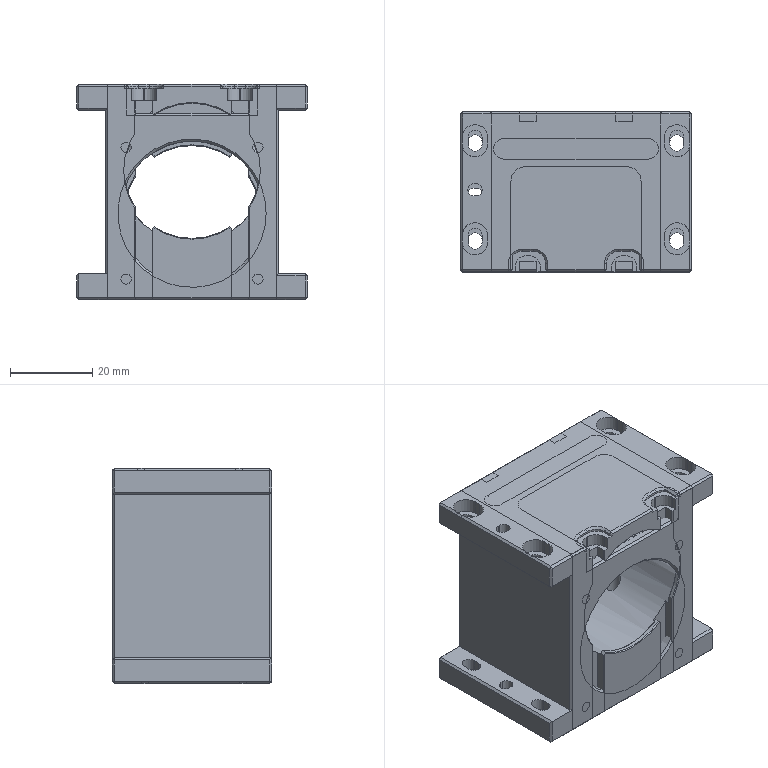NC program | NX | posted with a generic post | part box 56 x 38.8 x 52.3 mm
Lines 19 to 900 of 18366:
(外形动态铣 , TOOL : 粗刀D16)
N36 T18 M6
N38 G54
N40 G17 G0 G90 X-41.564 Y0.023 S8500 M3
N42 G43 Z22.1 H18
N44 G94 G1 Z-32.9 F5000.
N46 Z-35.9 F1300.
N48 X-40.3 Y-0.721 F4500.
N50 G3 X-37.96 Y0.142 R1.604
N52 X-37.568 Y1.641 R8.038
N54 X-37.25 Y4.662 R24.994
N56 X-37.043 Y10.905 R111.082
N58 X-37. Y19.341 R873.256
N60 G2 X-36.613 Y21.927 R8.763
N62 X-34.304 Y25.44 R8.355
N64 X-30.832 Y27.628 R11.747
N66 X-27.115 Y28.719 R18.953
N68 X-23.398 Y29.198 R31.73
N70 X-17.404 Y29.443 R97.007
N72 X-6.155 Y29.499 R760.069
N74 G1 X26.838 Y29.496
N76 G2 X29.424 Y29.11 R8.742
N78 X32.502 Y27.25 R8.354
N80 X34.595 Y24.465 R10.578
N82 X35.768 Y21.519 R15.001
N84 G1 X35.802 Y21.423
N86 X35.957 Y20.88
N88 G2 X36.666 Y16.315 R29.765
N90 X36.937 Y10.197 R90.363
N92 X36.997 Y-0.803 R751.906
N94 G1 X36.996 Y-19.328
N96 G2 X36.613 Y-21.915 R8.781
N98 X34.309 Y-25.431 R8.349
N100 X30.954 Y-27.574 R11.699
N102 X27.24 Y-28.693 R18.363
N104 X23.774 Y-29.166 R29.163
N106 X18.031 Y-29.431 R85.274
N108 X7.532 Y-29.498 R592.47
N110 G1 X-26.687
N112 G2 X-29.281 Y-29.157 R9.205
N114 X-32.483 Y-27.268 R8.278
N116 X-34.523 Y-24.597 R10.491
N118 X-35.758 Y-21.549 R15.048
N120 G1 X-35.781 Y-21.487
N122 X-35.941 Y-20.944
N124 G2 X-36.649 Y-16.505 R29.042
N126 X-36.933 Y-10.388 R85.934
N128 X-36.981 Y-4.138 R313.164
N130 X-36.753 Y-0.897 R42.178
N132 G3 X-36.2 Y6.624 R120.873
N134 G1 Y18.707
N136 G2 X-33.89 Y24.605 R8.272
N138 X-32.665 Y25.769 R17.702
N140 X-28.458 Y27.544 R8.274
N142 X-19.246 Y28.334 R84.093
N144 X-11.748 Y28.476 R284.478
N146 X-6.498 Y28.495 R400.209
N148 G1 X23.456 Y28.499
N150 G2 X27.72 Y27.678 R10.385
N152 G3 X28.15 Y27.571 R2.343
N154 G2 X33.271 Y25.225 R8.221
N156 X34.308 Y24.139 R16.303
N158 X35.802 Y21.423 R8.381
N160 G1 X35.957 Y20.88
N162 G2 X36.2 Y18.707 R8.323
N164 G1 Y-18.772
N166 G2 X33.75 Y-24.747 R8.238
N168 X32.585 Y-25.833 R13.123
N170 X28.575 Y-27.529 R8.313
N172 X19.115 Y-28.339 R84.949
N174 X9.116 Y-28.486 R322.982
N176 G1 X-1.384 Y-28.499
N178 X-23.456
N180 G2 X-27.72 Y-27.678 R10.379
N182 G3 X-28.219 Y-27.564 R2.143
N184 G2 X-33.205 Y-25.29 R8.208
N186 X-34.254 Y-24.203 R18.256
N188 X-35.781 Y-21.487 R8.364
N190 G3 X-33.75 Y-24.747 R8.305
N192 X-32.585 Y-25.833 R13.545
N194 X-28.219 Y-27.564 R8.218
N196 X-27.372 Y-27.6 R7.764
N198 G1 X27.489
N200 G3 X28.575 Y-27.529 R8.181
N202 G2 X30.152 Y-29.858 R1.6
N204 G1 X30.1 Y-29.951 Z-35.881
N206 X30.042 Y-30.04 Z-35.862
N208 X29.978 Y-30.126 Z-35.843
N210 X29.908 Y-30.206 Z-35.824
N212 X29.834 Y-30.282 Z-35.805
N214 X29.754 Y-30.353 Z-35.786
N216 X29.67 Y-30.418 Z-35.767
N218 X29.581 Y-30.477 Z-35.748
N220 X29.489 Y-30.531 Z-35.729
N222 X29.394 Y-30.578 Z-35.71
N224 X29.295 Y-30.619 Z-35.691
N226 X29.194 Y-30.653 Z-35.672
N228 X27.738 Y-31.092 Z-35.4
N230 X24.308 Y-32.124 F15000.
N232 X24.123 Y-32.154
N234 X23.937 Y-32.168
N236 X-34.297 Y-32.164
N238 G2 X-36.109 Y-30.883 R2.11
N240 G1 X-37.679 Y-27.176
N242 G2 X-37.656 Y-26.072 R1.604
N244 G1 X-37.517 Y-25.716
N246 X-36.496 Y-23.108 Z-35.9 F4500.
N248 X-36.013 Y-21.873
N250 G3 X-35.941 Y-20.944 R1.6
N252 G2 X-36.2 Y-18.772 R8.239
N254 G1 Y18.707
N256 G2 X-33.89 Y24.605 R8.272
N258 X-32.665 Y25.769 R17.702
N260 X-28.458 Y27.544 R8.274
N262 X-27.372 Y27.6 R8.406
N264 G1 X-13.792 Y27.599
N266 X-13.293 Y27.576
N268 G3 X-10.533 Y27.535 R143.585
N270 G2 X-9.447 Y27.6 R8.232
N272 G1 X9.564 Y27.599
N274 X10.107 Y27.577
N276 G3 X12.93 Y27.539 R121.082
N278 G2 X13.91 Y27.6 R8.154
N280 G1 X27.489
N282 G2 X28.157 Y27.57 R11.055
N284 G3 X27.489 Y27.6 R11.055
N286 G1 X13.91
N288 G3 X12.93 Y27.539 R8.154
N290 X11.963 Y27.372 R9.767
N292 G2 X11.194 Y27.423 R1.844
N294 G3 X10.107 Y27.577 R8.138
N296 G2 X8.882 Y28.386 R1.6
N298 G1 X8.695 Y28.721
N300 X7.561 Y30.74 Z-35.486
N302 X7.506 Y30.82 Z-35.469
N304 X7.447 Y30.896 Z-35.452
N306 X7.383 Y30.969 Z-35.435
N308 X7.314 Y31.037 Z-35.417
N310 X7.242 Y31.102 Z-35.4
N312 G3 X6.209 Y31.475 R1.604 F15000.
N314 G1 X-6.739 Y31.429
N316 G3 X-7.6 Y31.105 R1.608
N318 G1 X-7.685 Y31.035 Z-35.42 F4500.
N320 X-7.765 Y30.96 Z-35.439
N322 X-7.84 Y30.879 Z-35.459
N324 X-7.909 Y30.794 Z-35.479
N326 X-7.972 Y30.704 Z-35.498
N328 X-8.029 Y30.609 Z-35.518
N330 X-9.068 Y28.739 Z-35.9
N332 X-9.283 Y28.351
N334 G2 X-10.533 Y27.535 R1.6
N336 G3 X-11.433 Y27.374 R10.764
N338 G2 X-12.163 Y27.414 R1.894
N340 G3 X-13.374 Y27.58 R7.722
N342 G2 X-14.908 Y29.042 R1.616
N344 G1 X-15.103 Y31.099
N346 Z-32.9
N348 G0 Z22.1
N350 X17.252 Y-31.102
N352 G1 Z-3.9 F5000.
N354 Z-6.9 F1300.
N356 X16.894 Y-28.941 F4500.
N358 G3 X15.405 Y-27.592 R1.616
N360 G2 X13.667 Y-27.318 R7.505
N362 G3 X10.793 Y-26.898 R19.685
N364 X4.995 Y-26.658 R90.989
N366 X-6.906 Y-26.599 R799.149
N368 G1 X-11.408 Y-26.601
N370 G3 X-12.179 Y-26.762 R1.949
N372 G2 X-15.376 Y-27.593 R8.165
N374 G3 X-12.179 Y-26.762 R8.165
N376 G1 X-12.16 Y-26.754
N378 X-11.941 Y-26.634
N380 G2 X-11.302 Y-26.399 R3.71
N382 X-8.697 Y-25.956 R15.438
N384 X-3.492 Y-25.686 R66.802
N386 X7.27 Y-25.752 R197.849
N388 X10.569 Y-25.986 R47.826
N390 X11.295 Y-26.255 R1.957
N392 G3 X13.727 Y-27.334 R8.193
N394 G2 X11.295 Y-26.255 R8.193
N396 G1 X11.191 Y-26.188
N398 X11.09 Y-26.114
N400 G3 X10.692 Y-25.892 R2.029
N402 X8.789 Y-25.331 R9.301
N404 X4.818 Y-24.87 R32.163
N406 X-6.184 Y-24.848 R99.505
N408 X-9.423 Y-25.208 R27.725
N410 X-10.275 Y-25.501 R2.207
N412 G1 X-10.507 Y-25.668
N414 G2 X-11.947 Y-26.638 R7.635
N416 G3 X-10.507 Y-25.668 R7.635
N418 G1 X-10.228 Y-25.417
N420 G2 X-9.095 Y-24.851 R4.546
N422 X-6.504 Y-24.238 R14.083
N424 X-1.79 Y-23.855 R40.947
N426 X5.385 Y-24.017 R62.847
N428 X8.725 Y-24.533 R21.992
N430 X9.443 Y-24.77 R3.308
N432 X9.882 Y-25.084 R2.112
N434 G3 X11.115 Y-26.133 R8.87
N436 G2 X9.882 Y-25.084 R8.87
N438 G1 X9.603 Y-24.806
N440 G3 X8.539 Y-24.192 R4.366
N442 X6.087 Y-23.488 R12.475
N444 X1.785 Y-23.02 R30.841
N446 X-4.81 Y-23.179 R44.497
N448 X-7.847 Y-23.73 R18.933
N450 X-8.718 Y-24.029 R5.421
N452 X-9.237 Y-24.42 R2.064
N454 G2 X-10.277 Y-25.461 R15.115
N456 G3 X-9.237 Y-24.42 R15.115
N458 G1 X-9.042 Y-24.207
N460 G2 X-8.727 Y-23.92 R1.791
N462 X-7.163 Y-23.139 R6.261
N464 X-4.087 Y-22.432 R15.885
N466 X4.41 Y-22.41 R33.677
N468 X7.539 Y-23.106 R16.182
N470 X8.261 Y-23.41 R4.293
N472 X8.76 Y-23.846 R2.051
N474 G1 X9.042 Y-24.207
N476 X9.635 Y-24.838
N478 X9.017 Y-24.177
N480 X8.619 Y-23.663
N482 G3 X8.326 Y-23.345 R1.707
N484 X7.008 Y-22.563 R5.333
N486 X4.166 Y-21.745 R12.963
N488 X-4.378 Y-21.691 R26.543
N490 X-7.206 Y-22.457 R13.282
N492 X-7.822 Y-22.753 R4.324
N494 X-8.365 Y-23.284 R1.971
N496 G1 X-8.619 Y-23.663
N498 X-8.9 Y-24.034
N500 X-9.042 Y-24.207
N502 X-8.9 Y-24.034
N504 X-8.619 Y-23.663
N506 X-8.356 Y-23.271
N508 X-8.263 Y-23.119
N510 G2 X-8.006 Y-22.78 R1.688
N512 X-6.962 Y-22.036 R4.512
N514 X-4.693 Y-21.19 R10.297
N516 X-0.126 Y-20.634 R19.833
N518 X4.588 Y-21.079 R20.914
N520 X7.063 Y-21.915 R10.915
N522 X7.663 Y-22.282 R3.214
N524 X8.08 Y-22.787 R2.061
N526 G1 X8.263 Y-23.12
N528 X8.474 Y-23.452
N530 X8.619 Y-23.663
N532 X8.474 Y-23.452
N534 X8.263 Y-23.12
N536 X7.965 Y-22.576
N538 X7.93 Y-22.507
N540 X7.869 Y-22.398
N542 G3 X6.968 Y-21.584 R3.545
N544 X4.809 Y-20.608 R8.607
N546 X0.856 Y-19.945 R16.359
N548 X-4.383 Y-20.393 R18.389
N550 X-6.883 Y-21.345 R9.757
N552 X-7.453 Y-21.753 R2.787
N554 X-7.821 Y-22.273 R2.078
N556 G1 X-7.964 Y-22.576
N558 X-8.263 Y-23.119
N560 X-7.964 Y-22.576
N562 X-7.813 Y-22.256
N564 X-7.716 Y-22.032
N566 X-7.666 Y-21.918
N568 G2 X-7.027 Y-21.198 R2.949
N570 X-5.236 Y-20.167 R6.793
N572 X-1.759 Y-19.333 R13.356
N574 X3.88 Y-19.653 R16.865
N576 X6.34 Y-20.564 R10.041
N578 X7.158 Y-21.104 R5.023
N580 X7.623 Y-21.781 R1.928
N582 G1 X7.716 Y-22.033
N584 X7.93 Y-22.507
N586 X7.716 Y-22.033
N588 X7.514 Y-21.489
N590 X7.467 Y-21.374
N592 G3 X6.862 Y-20.641 R3.036
N594 X4.991 Y-19.505 R6.721
N596 X1.35 Y-18.636 R12.655
N598 X-3.979 Y-19.066 R14.963
N600 X-6.337 Y-20.07 R9.067
N602 X-7.024 Y-20.588 R4.103
N604 X-7.474 Y-21.353 R1.935
N606 G1 X-7.514 Y-21.489
N608 X-7.716 Y-22.032
N610 X-7.514 Y-21.489
N612 X-7.354 Y-20.945
N614 G2 X-6.809 Y-20.168 R2.748
N616 X-5.315 Y-19.101 R5.958
N618 X-2.402 Y-18.147 R10.402
N620 X3.793 Y-18.422 R13.834
N622 X6.285 Y-19.56 R8.605
N624 X6.962 Y-20.135 R3.725
N626 X7.339 Y-20.879 R1.921
N628 G1 X7.354 Y-20.946
N630 X7.387 Y-21.069
N632 X7.514 Y-21.489
N634 X7.387 Y-21.069
N636 X7.354 Y-20.946
N638 X7.258 Y-20.513
N640 X7.222 Y-20.393
N642 G3 X6.679 Y-19.602 R2.926
N644 X5.243 Y-18.529 R5.938
N646 X2.324 Y-17.521 R9.94
N648 X-3.847 Y-17.852 R12.805
N650 X-5.983 Y-18.86 R8.375
N652 X-6.873 Y-19.622 R4.509
N654 X-7.233 Y-20.402 R1.907
N656 G1 X-7.269 Y-20.582
N658 X-7.354 Y-20.945
N660 X-7.269 Y-20.582
N662 X-7.233 Y-20.402
N664 X-7.196 Y-20.155
N666 G2 X-7.062 Y-19.74 R1.719
N668 X-6.315 Y-18.777 R3.464
N670 X-4.274 Y-17.506 R6.927
N672 X-0.678 Y-16.706 R11.076
N674 X3.943 Y-17.315 R11.871
N676 X6.071 Y-18.427 R7.943
N678 X6.799 Y-19.099 R4.758
N680 X7.162 Y-19.93 R1.921
N682 G1 X7.234 Y-20.402
N684 X7.261 Y-20.524
N686 X7.234 Y-20.402
N688 X7.151 Y-19.859
N690 X7.141 Y-19.734
N692 X7.101 Y-19.487
N694 G3 X6.663 Y-18.687 R2.739
N696 X5.298 Y-17.49 R5.277
N698 X2.318 Y-16.327 R9.092
N700 X-3.376 Y-16.556 R11.721
N702 X-5.783 Y-17.708 R8.26
N704 X-6.755 Y-18.601 R5.171
N706 X-7.125 Y-19.548 R1.872
N708 G1 X-7.151 Y-19.858
N710 X-7.207 Y-20.229
N712 X-7.151 Y-19.858
N714 X-7.105 Y-19.315
N716 X-7.08 Y-19.066
N718 G2 X-6.659 Y-18.212 R2.658
N720 X-5.299 Y-16.955 R5.201
N722 X-2.302 Y-15.74 R8.86
N724 X3.52 Y-16.035 R11.235
N726 X5.9 Y-17.284 R7.909
N728 X6.807 Y-18.205 R4.745
N730 X7.103 Y-19.168 R1.878
N732 G1 X7.105 Y-19.315
N734 X7.147 Y-19.813
N736 X7.105 Y-19.315
N738 X7.095 Y-18.772
N740 X7.083 Y-18.647
N742 G3 X6.697 Y-17.777 R2.641
N744 X5.351 Y-16.454 R5.131
N746 X2.411 Y-15.188 R8.529
N748 X-3.562 Y-15.486 R10.897
N750 X-5.912 Y-16.776 R7.675
N752 X-6.822 Y-17.759 R4.776
N754 X-7.095 Y-18.723 R1.881
N756 G1 Y-18.772
N758 X-7.105 Y-19.315
N760 X-7.095 Y-18.772
N762 Y-18.348
N764 G2 X-7.016 Y-17.923 R1.7
N766 X-6.232 Y-16.677 R3.637
N768 X-4.007 Y-15.153 R6.925
N770 X0.486 Y-14.339 R10.228
N772 X4.452 Y-15.302 R9.96
N774 X6.417 Y-16.734 R6.709
N776 X6.894 Y-17.369 R3.386
N778 X7.095 Y-18.168 R1.926
N780 G1 Y-18.772
N782 Y-17.793
N784 X7.085 Y-17.668
N786 G3 X6.577 Y-16.57 R3.006
N788 X5.198 Y-15.262 R5.703
N790 X2.296 Y-14.022 R8.481
N792 X-3.698 Y-14.417 R10.413
N794 X-5.998 Y-15.791 R7.47
N796 X-6.849 Y-16.769 R5.038
N798 X-7.095 Y-17.658 R1.912
N800 G1 Y-18.408
N802 Y-17.283
N804 X-7.086 Y-17.158
N806 G2 X-6.723 Y-16.266 R2.895
N808 X-5.435 Y-14.889 R5.125
N810 X-2.767 Y-13.581 R8.034
N812 X3.735 Y-13.873 R10.248
N814 X6.059 Y-15.307 R7.524
N816 X6.82 Y-16.193 R5.311
N818 X7.095 Y-17.16 R1.879
N820 G1 Y-17.91
N822 Y-16.785
N824 X7.088 Y-16.66
N826 G3 X6.739 Y-15.758 R2.776
N828 X5.516 Y-14.402 R5.015
N830 X2.918 Y-13.063 R7.898
N832 X-3.904 Y-13.387 R10.111
N834 X-6.151 Y-14.854 R7.397
N836 X-6.868 Y-15.741 R4.746
N838 X-7.095 Y-16.611 R1.926
N840 G1 Y-17.361
N842 Y-16.236
N844 G2 X-7.017 Y-15.819 R1.701
N846 X-6.417 Y-14.743 R3.503
N848 X-4.803 Y-13.351 R6.309
N850 X-1.389 Y-12.159 R8.983
N852 X3.717 Y-12.751 R10.067
N854 X5.998 Y-14.16 R7.573
N856 X6.86 Y-15.192 R4.918
N858 X7.095 Y-16.068 R1.92
N860 G1 Y-16.818
N862 Y-15.693
N864 X7.088 Y-15.569
N866 G3 X6.735 Y-14.663 R2.908
N868 X5.5 Y-13.287 R5.115
N870 X2.406 Y-11.797 R8.161
N872 X-3.644 Y-12.165 R10.014
N874 X-5.974 Y-13.59 R7.607
N876 X-6.846 Y-14.618 R5.003
N878 X-7.095 Y-15.51 R1.91
N880 G1 Y-16.26
N882 Y-15.135
N884 G2 X-7.016 Y-14.721 R1.686
N886 X-6.261 Y-13.453 R3.838
N888 X-4.12 Y-11.86 R6.809
N890 X0.552 Y-10.946 R9.632
N892 X4.579 Y-12.047 R9.404
N894 X6.514 Y-13.609 R6.564
N896 X6.897 Y-14.159 R3.572
N898 X7.095 Y-14.953 R1.931
N900 G1 Y-15.703
N902 Y-14.578
N904 G3 X6.815 Y-13.708 R2.517
N906 X5.596 Y-12.254 R5.058
N908 X2.894 Y-10.815 R7.853
N910 X-3.934 Y-11.169 R9.869
N912 X-6.152 Y-12.65 R7.256
N914 X-6.875 Y-13.56 R4.882
N916 X-7.095 Y-14.425 R1.931
N918 G1 Y-15.175
N920 Y-14.05
N922 X-7.088 Y-13.925
N924 G2 X-6.738 Y-13.013 R2.9
N926 X-5.497 Y-11.618 R5.136
N928 X-2.552 Y-10.155 R8.089
N930 X3.977 Y-10.63 R9.855
N932 X6.121 Y-12.068 R7.251
N934 X6.851 Y-12.969 R5.203
N936 X7.095 Y-13.855 R1.913
N938 G1 Y-14.605
N940 Y-13.48
N942 X7.087 Y-13.355
N944 G3 X6.733 Y-12.451 R2.985
N946 X5.484 Y-11.052 R5.2
N948 X2.533 Y-9.592 R8.126
N950 X-4.017 Y-10.092 R9.81
N952 X-6.228 Y-11.621 R7.206
N954 X-6.848 Y-12.402 R5.496
N956 X-7.095 Y-13.291 R1.911
N958 G1 Y-14.166
N960 Y-12.916
N962 X-7.086 Y-12.792
N964 G2 X-6.621 Y-11.708 R3.092
N966 X-5.067 Y-10.181 R5.789
N968 X-1.602 Y-8.828 R8.682
N970 X4.064 Y-9.556 R9.793
N972 X6.247 Y-11.085 R7.233
N974 X6.875 Y-11.897 R5.133
N976 X7.095 Y-12.761 R1.932
N978 G1 Y-13.511
N980 Y-12.386
N982 G3 X7.013 Y-11.954 R1.727
N984 X6.243 Y-10.658 R3.884
N986 X3.898 Y-8.965 R7.055
N988 X-4.009 Y-8.97 R9.735
N990 X-6.227 Y-10.504 R7.189
N992 X-6.844 Y-11.281 R5.521
N994 X-7.095 Y-12.174 R1.909
N996 G1 Y-12.924
N998 Y-11.799
N1000 X-7.086 Y-11.674
N1002 G2 X-6.621 Y-10.592 R3.098
N1004 X-5.066 Y-9.062 R5.806
N1006 X-1.823 Y-7.749 R8.613
N1008 X4.154 Y-8.482 R9.744
N1010 X6.333 Y-10.064 R7.12
N1012 X6.908 Y-10.85 R4.169
N1014 X7.095 Y-11.628 R1.94
N1016 G1 Y-12.503
N1018 Y-11.253
N1020 G3 X7.016 Y-10.841 R1.718
N1022 X6.244 Y-9.543 R3.922
N1024 X3.895 Y-7.847 R7.08
N1026 X-1.443 Y-7.112 R9.701
N1028 X-5.036 Y-8.412 R8.905
N1030 X-6.625 Y-9.855 R6.175
N1032 X-6.976 Y-10.456 R2.573
N1034 X-7.095 Y-11.094 R2.066
N1036 G1 Y-11.844
N1038 Y-10.719
N1040 X-7.089 Y-10.594
N1042 G2 X-6.617 Y-9.472 R3.049
N1044 X-5.064 Y-7.944 R5.825
N1046 X-1.75 Y-6.617 R8.655
N1048 X3.857 Y-7.228 R9.836
N1050 X6.122 Y-8.726 R7.476
N1052 X6.849 Y-9.622 R5.298
N1054 X7.095 Y-10.51 R1.912
N1056 G1 Y-11.26
N1058 Y-10.135
N1060 G3 X7.015 Y-9.721 R1.719
N1062 X6.244 Y-8.426 R3.927
N1064 X3.896 Y-6.73 R7.074
N1066 X-4.039 Y-6.748 R9.739
N1068 X-6.26 Y-8.307 R7.156
N1070 X-6.866 Y-9.088 R5.201
N1072 X-7.095 Y-9.959 R1.924
N1074 G1 Y-10.834
N1076 Y-9.584
N1078 X-7.087 Y-9.46
N1080 G2 X-6.737 Y-8.555 R2.962
N1082 X-5.488 Y-7.148 R5.226
N1084 X-2.687 Y-5.722 R7.985
N1086 X4.139 Y-6.24 R9.763
N1088 X6.373 Y-7.877 R7.124
N1090 X6.874 Y-8.552 R4.357
N1092 X7.095 Y-9.417 R1.93
N1094 G1 Y-10.167
N1096 Y-9.042
N1098 X7.088 Y-8.917
N1100 G3 X6.762 Y-8.042 R2.77
N1102 X5.529 Y-6.626 R5.278
N1104 X2.743 Y-5.18 R7.962
N1106 X-4.088 Y-5.656 R9.775
N1108 X-6.256 Y-7.188 R7.221
N1110 X-6.866 Y-7.973 R5.235
N1112 X-7.095 Y-8.844 R1.924
N1114 G1 Y-9.594
N1116 Y-8.469
N1118 G2 X-7.019 Y-8.06 R1.689
N1120 X-6.421 Y-6.968 R3.626
N1122 X-4.655 Y-5.452 R6.411
N1124 X-0.695 Y-4.248 R9.104
N1126 X4.23 Y-5.167 R9.637
N1128 X6.409 Y-6.803 R7.032
N1130 X6.893 Y-7.477 R3.8
N1132 X7.095 Y-8.277 R1.925
N1134 G1 Y-9.152
N1136 Y-7.902
N1138 G3 X7.014 Y-7.488 R1.686
N1140 X6.242 Y-6.193 R3.945
N1142 X3.896 Y-4.495 R7.053
N1144 X-0.833 Y-3.713 R9.465
N1146 X-4.09 Y-4.549 R9.788
N1148 X-6.255 Y-6.073 R7.193
N1150 X-6.864 Y-6.854 R5.238
N1152 X-7.095 Y-7.726 R1.922
N1154 G1 Y-8.476
N1156 Y-7.351
N1158 G2 X-7.019 Y-6.944 R1.686
N1160 X-6.417 Y-5.85 R3.602
N1162 X-4.759 Y-4.409 R6.369
N1164 X-1.658 Y-3.268 R9.022
N1166 X3.944 Y-3.919 R9.648
N1168 X6.208 Y-5.466 R7.297
N1170 X6.894 Y-6.359 R4.551
N1172 X7.095 Y-7.158 R1.926
N1174 G1 Y-7.908
N1176 Y-6.783
N1178 G3 X7.013 Y-6.368 R1.685
N1180 X6.245 Y-5.079 R3.934
N1182 X3.831 Y-3.353 R7.073
N1184 X0.947 Y-2.605 R9.131
N1186 G1 X-0.428
N1188 G3 X-4.469 Y-3.634 R9.221
N1190 X-6.389 Y-5.114 R6.943
N1192 X-6.905 Y-5.835 R3.899
N1194 X-7.095 Y-6.617 R1.938
N1196 G1 Y-7.367
N1198 Y-6.242
N1200 G2 X-7.018 Y-5.832 R1.69
N1202 X-6.409 Y-4.735 R3.597
N1204 X-4.782 Y-3.319 R6.358
N1206 X-3.494 Y-2.687 R7.001
N1208 X-2.972 Y-2.605 R2.124
N1210 G1 X-0.347
N1212 X-3.472
N1214 G3 X-4.972 Y-3.064 R4.253
N1216 X-6.812 Y-4.65 R5.009
N1218 X-7.095 Y-5.621 R1.874
N1220 G1 Y-6.246
N1222 Y-5.246
N1224 G2 X-7.017 Y-4.833 R1.682
N1226 X-6.179 Y-3.541 R3.462
N1228 X-5.215 Y-2.808 R4.56
N1230 X-4.415 Y-2.605 R1.926
N1232 G1 X-3.415
N1234 X-4.79
N1236 G3 X-5.212 Y-2.686 R1.729
N1238 X-6.752 Y-3.773 R3.352
N1240 X-7.095 Y-4.778 R1.851
N1242 G1 Y-5.278
N1244 Y-4.528
N1246 X-7.076 Y-4.278
N1248 G2 X-6.674 Y-3.436 R2.216
N1250 X-6.184 Y-2.94 R2.902
N1252 X-5.219 Y-2.605 R1.984
N1254 G1 X-4.719
N1256 X-5.219
N1258 G3 X-6.069 Y-2.732 R1.98
N1260 X-7.095 Y-4.268 R1.662
N1262 G1 Y-4.643
N1264 G2 X-7.063 Y-3.943 R3.571
N1266 X-5.432 Y-2.605 R1.662
N1268 G1 X2.322
N1270 G2 X4.869 Y-3.395 R6.177
N1272 X6.819 Y-5.147 R5.783
N1274 X7.095 Y-6.115 R1.879
N1276 G1 Y-6.865
N1278 Y-5.74
N1280 X7.088 Y-5.615
N1282 G3 X6.74 Y-4.715 R2.757
N1284 X5.223 Y-3.166 R4.975
N1286 X4.357 Y-2.701 R4.218
N1288 X3.806 Y-2.605 R2.092
N1290 G1 X2.306
N1292 X4.181
N1294 G2 X4.628 Y-2.676 R2.015
N1296 X6.844 Y-4.288 R3.983
N1298 X7.095 Y-5.165 R1.919
N1300 G1 Y-5.79
N1302 Y-4.915
N1304 X7.081 Y-4.665
N1306 G3 X6.705 Y-3.806 R2.452
N1308 X5.738 Y-2.859 R3.536
N1310 X4.858 Y-2.605 R1.918
N1312 G1 X4.108
N1314 X5.108
N1316 X5.358 Y-2.619
N1318 G2 X6.449 Y-3.183 R2.511
N1320 X7.037 Y-4.119 R1.705
N1322 G1 X7.095 Y-4.459
N1324 Y-4.959
N1326 Y-4.459
N1328 G3 X6.815 Y-3.344 R1.83
N1330 X5.432 Y-2.605 R1.662
N1332 G1 X5.057
N1334 G3 X3.46 Y-3.977 R1.616
N1336 G1 X3.134 Y-6.105
N1338 Z-3.9
N1340 G0 Z22.1
N1342 X-41.564 Y0.023
N1344 G1 Z-50.9 F5000.
N1346 Z-53.9 F1300.
N1348 X-40.3 Y-0.721 F4500.
N1350 G3 X-37.96 Y0.142 R1.604
N1352 X-37.568 Y1.641 R8.038
N1354 X-37.25 Y4.662 R24.994
N1356 X-37.043 Y10.905 R111.082
N1358 X-37. Y19.341 R873.256
N1360 G2 X-36.613 Y21.927 R8.763
N1362 X-34.304 Y25.44 R8.355
N1364 X-30.832 Y27.628 R11.747
N1366 X-27.115 Y28.719 R18.953
N1368 X-23.398 Y29.198 R31.73
N1370 X-17.404 Y29.443 R97.007
N1372 X-6.155 Y29.499 R760.069
N1374 G1 X26.838 Y29.496
N1376 G2 X29.424 Y29.11 R8.742
N1378 X32.502 Y27.25 R8.354
N1380 X34.595 Y24.465 R10.578
N1382 X35.768 Y21.519 R15.001
N1384 G1 X35.802 Y21.423
N1386 X35.957 Y20.88
N1388 G2 X36.666 Y16.315 R29.765
N1390 X36.937 Y10.197 R90.363
N1392 X36.997 Y-0.803 R751.906
N1394 G1 X36.996 Y-19.328
N1396 G2 X36.613 Y-21.915 R8.781
N1398 X34.309 Y-25.431 R8.349
N1400 X30.954 Y-27.574 R11.699
N1402 X27.24 Y-28.693 R18.363
N1404 X23.774 Y-29.166 R29.163
N1406 X18.031 Y-29.431 R85.274
N1408 X7.532 Y-29.498 R592.47
N1410 G1 X-26.687
N1412 G2 X-29.281 Y-29.157 R9.205
N1414 X-32.483 Y-27.268 R8.278
N1416 X-34.523 Y-24.597 R10.491
N1418 X-35.758 Y-21.549 R15.048
N1420 G1 X-35.781 Y-21.487
N1422 X-35.941 Y-20.944
N1424 G2 X-36.649 Y-16.505 R29.042
N1426 X-36.933 Y-10.388 R85.934
N1428 X-36.981 Y-4.138 R313.164
N1430 X-36.753 Y-0.897 R42.178
N1432 G3 X-36.2 Y6.624 R120.873
N1434 G1 Y18.707
N1436 G2 X-33.89 Y24.605 R8.272
N1438 X-32.665 Y25.769 R17.702
N1440 X-28.458 Y27.544 R8.274
N1442 X-19.246 Y28.334 R84.093
N1444 X-11.748 Y28.476 R284.478
N1446 X-6.498 Y28.495 R400.209
N1448 G1 X23.456 Y28.499
N1450 G2 X27.72 Y27.678 R10.385
N1452 G3 X28.15 Y27.571 R2.343
N1454 G2 X33.271 Y25.225 R8.221
N1456 X34.308 Y24.139 R16.303
N1458 X35.802 Y21.423 R8.381
N1460 G1 X35.957 Y20.88
N1462 G2 X36.2 Y18.707 R8.323
N1464 G1 Y-18.772
N1466 G2 X33.75 Y-24.747 R8.238
N1468 X32.585 Y-25.833 R13.123
N1470 X28.575 Y-27.529 R8.313
N1472 X19.115 Y-28.339 R84.949
N1474 X9.116 Y-28.486 R322.982
N1476 G1 X-1.384 Y-28.499
N1478 X-23.456
N1480 G2 X-27.72 Y-27.678 R10.379
N1482 G3 X-28.219 Y-27.564 R2.143
N1484 G2 X-33.205 Y-25.29 R8.208
N1486 X-34.254 Y-24.203 R18.256
N1488 X-35.781 Y-21.487 R8.364
N1490 G3 X-33.75 Y-24.747 R8.305
N1492 X-32.585 Y-25.833 R13.545
N1494 X-28.219 Y-27.564 R8.218
N1496 X-27.372 Y-27.6 R7.764
N1498 G1 X27.489
N1500 G3 X28.575 Y-27.529 R8.181
N1502 G2 X30.152 Y-29.858 R1.6
N1504 G1 X30.1 Y-29.951 Z-53.881
N1506 X30.042 Y-30.04 Z-53.862
N1508 X29.978 Y-30.126 Z-53.843
N1510 X29.908 Y-30.206 Z-53.824
N1512 X29.834 Y-30.282 Z-53.805
N1514 X29.754 Y-30.353 Z-53.786
N1516 X29.67 Y-30.418 Z-53.767
N1518 X29.581 Y-30.477 Z-53.748
N1520 X29.489 Y-30.531 Z-53.729
N1522 X29.394 Y-30.578 Z-53.71
N1524 X29.295 Y-30.619 Z-53.691
N1526 X29.194 Y-30.653 Z-53.672
N1528 X27.738 Y-31.092 Z-53.4
N1530 X24.308 Y-32.124 F15000.
N1532 X24.123 Y-32.154
N1534 X23.937 Y-32.168
N1536 X-34.297 Y-32.164
N1538 G2 X-36.109 Y-30.883 R2.11
N1540 G1 X-37.679 Y-27.176
N1542 G2 X-37.656 Y-26.072 R1.604
N1544 G1 X-37.517 Y-25.716
N1546 X-36.496 Y-23.108 Z-53.9 F4500.
N1548 X-36.013 Y-21.873
N1550 G3 X-35.941 Y-20.944 R1.6
N1552 G2 X-36.2 Y-18.772 R8.239
N1554 G1 Y18.707
N1556 G2 X-33.89 Y24.605 R8.272
N1558 X-32.665 Y25.769 R17.702
N1560 X-28.458 Y27.544 R8.274
N1562 X-27.372 Y27.6 R8.406
N1564 G1 X-13.792 Y27.599
N1566 X-13.293 Y27.576
N1568 G3 X-10.533 Y27.535 R143.585
N1570 G2 X-9.447 Y27.6 R8.232
N1572 G1 X9.564 Y27.599
N1574 X10.107 Y27.577
N1576 G3 X12.93 Y27.539 R121.082
N1578 G2 X13.91 Y27.6 R8.154
N1580 G1 X27.489
N1582 G2 X28.157 Y27.57 R11.055
N1584 G3 X27.489 Y27.6 R11.055
N1586 G1 X13.91
N1588 G3 X12.93 Y27.539 R8.154
N1590 X11.963 Y27.372 R9.767
N1592 G2 X11.194 Y27.423 R1.844
N1594 G3 X10.107 Y27.577 R8.138
N1596 G2 X8.882 Y28.386 R1.6
N1598 G1 X8.695 Y28.721
N1600 X7.561 Y30.74 Z-53.486
N1602 X7.506 Y30.82 Z-53.469
N1604 X7.447 Y30.896 Z-53.452
N1606 X7.383 Y30.969 Z-53.435
N1608 X7.314 Y31.037 Z-53.417
N1610 X7.242 Y31.102 Z-53.4
N1612 G3 X6.209 Y31.475 R1.604 F15000.
N1614 G1 X-6.739 Y31.429
N1616 G3 X-7.6 Y31.105 R1.608
N1618 G1 X-7.685 Y31.035 Z-53.42 F4500.
N1620 X-7.765 Y30.96 Z-53.439
N1622 X-7.84 Y30.879 Z-53.459
N1624 X-7.909 Y30.794 Z-53.479
N1626 X-7.972 Y30.704 Z-53.498
N1628 X-8.029 Y30.609 Z-53.518
N1630 X-9.068 Y28.739 Z-53.9
N1632 X-9.283 Y28.351
N1634 G2 X-10.533 Y27.535 R1.6
N1636 G3 X-11.433 Y27.374 R10.764
N1638 G2 X-12.163 Y27.414 R1.894
N1640 G3 X-13.374 Y27.58 R7.722
N1642 G2 X-14.908 Y29.042 R1.616
N1644 G1 X-15.103 Y31.099
N1646 Z-50.9
N1648 G0 Z22.1
(螺旋内圆D10 , TOOL : 粗刀D16)
N1650 G18 X0. Z-31.3 S7000
N1652 Y-52.5
N1654 Y-19.9
N1656 G41 G1 X0.017 Z-31.499 F2000. D18
N1658 G2 X4.65 Z-31.3 R2.321
N1660 X4.65 Y-18.9 Z-31.3 I-4.65 K0.
N1662 X4.65 Y-17.9 Z-31.3 I-4.65 K0.
N1664 X4.65 Y-16.9 Z-31.3 I-4.65 K0.
N1666 X4.65 Y-15.9 Z-31.3 I-4.65 K0.
N1668 X4.65 Y-14.9 Z-31.3 I-4.65 K0.
N1670 X4.65 Y-13.9 Z-31.3 I-4.65 K0.
N1672 X4.65 Y-12.9 Z-31.3 I-4.65 K0.
N1674 X4.65 Y-11.9 Z-31.3 I-4.65 K0.
N1676 X4.65 Y-10.9 Z-31.3 I-4.65 K0.
N1678 X4.65 Y-9.9 Z-31.3 I-4.65 K0.
N1680 X4.65 Y-8.9 Z-31.3 I-4.65 K0.
N1682 X4.65 Y-7.9 Z-31.3 I-4.65 K0.
N1684 X4.65 Y-6.9 Z-31.3 I-4.65 K0.
N1686 X4.65 Y-5.9 Z-31.3 I-4.65 K0.
N1688 X4.65 Y-4.9 Z-31.3 I-4.65 K0.
N1690 X4.65 Y-3.9 Z-31.3 I-4.65 K0.
N1692 X4.65 Y-2.9 Z-31.3 I-4.65 K0.
N1694 X4.65 Y-1.9 Z-31.3 I-4.65 K0.
N1696 X4.65 Y-0.9 Z-31.3 I-4.65 K0.
N1698 X4.65 Y0.1 Z-31.3 I-4.65 K0.
N1700 X4.65 Y1.1 Z-31.3 I-4.65 K0.
N1702 X4.65 Y2.1 Z-31.3 I-4.65 K0.
N1704 X4.65 Y3.1 Z-31.3 I-4.65 K0.
N1706 X4.65 Y4.1 Z-31.3 I-4.65 K0.
N1708 X4.65 Y5.1 Z-31.3 I-4.65 K0.
N1710 X4.65 Y6.1 Z-31.3 I-4.65 K0.
N1712 X4.65 Y7.1 Z-31.3 I-4.65 K0.
N1714 X4.65 Y8.1 Z-31.3 I-4.65 K0.
N1716 X4.65 Y9.1 Z-31.3 I-4.65 K0.
N1718 X4.65 Y10.1 Z-31.3 I-4.65 K0.
N1720 X4.65 Y11.1 Z-31.3 I-4.65 K0.
N1722 X4.65 Y12.1 Z-31.3 I-4.65 K0.
N1724 X4.65 Y13.1 Z-31.3 I-4.65 K0.
N1726 X4.65 Y14.1 Z-31.3 I-4.65 K0.
N1728 X4.65 Y15.1 Z-31.3 I-4.65 K0.
N1730 X4.65 Y16.1 Z-31.3 I-4.65 K0.
N1732 X4.65 Y17.1 Z-31.3 I-4.65 K0.
N1734 X4.422 Y18.05 Z-32.737 R-4.65
N1736 X1.437 Z-26.878 R4.65
N1738 X4.422 Z-32.737 R-4.65
N1740 X0.078 Z-31.116 R2.321
N1742 G40
N1744 G1 X0. Z-31.3
N1746 G0 Y-19.9
N1748 G41 G1 X0.009 Z-31.5
N1750 G2 X9.3 Z-31.3 R4.648
N1752 X9.3 Y-18.9 Z-31.3 I-9.3 K0.
N1754 X9.3 Y-17.9 Z-31.3 I-9.3 K0.
N1756 X9.3 Y-16.9 Z-31.3 I-9.3 K0.
N1758 X9.3 Y-15.9 Z-31.3 I-9.3 K0.
N1760 X9.3 Y-14.9 Z-31.3 I-9.3 K0.
N1762 X9.3 Y-13.9 Z-31.3 I-9.3 K0.
N1764 X9.3 Y-12.9 Z-31.3 I-9.3 K0.
N1766 X9.3 Y-11.9 Z-31.3 I-9.3 K0.
N1768 X9.3 Y-10.9 Z-31.3 I-9.3 K0.
N1770 X9.3 Y-9.9 Z-31.3 I-9.3 K0.
N1772 X9.3 Y-8.9 Z-31.3 I-9.3 K0.
N1774 X9.3 Y-7.9 Z-31.3 I-9.3 K0.
N1776 X9.3 Y-6.9 Z-31.3 I-9.3 K0.
N1778 X9.3 Y-5.9 Z-31.3 I-9.3 K0.
N1780 X9.3 Y-4.9 Z-31.3 I-9.3 K0.
N1782 X9.3 Y-3.9 Z-31.3 I-9.3 K0.
N1784 X9.3 Y-2.9 Z-31.3 I-9.3 K0.
N1786 X9.3 Y-1.9 Z-31.3 I-9.3 K0.